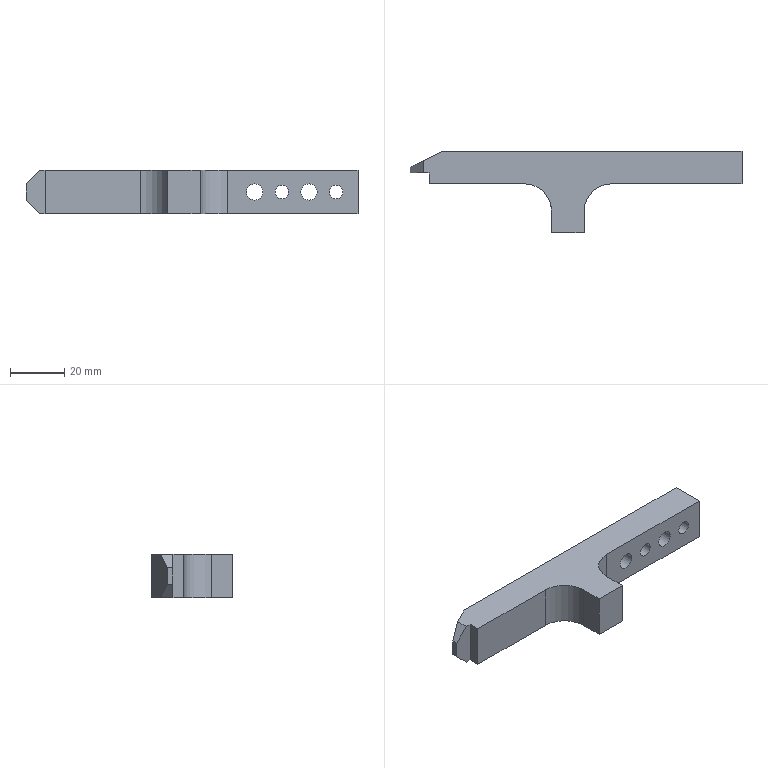Part | NX | features BREP 1 | 1 solid | 21 faces | box 122 x 30 x 16 mm | volume 25322 mm3 | plane 15 | cylinder 6 | commonest cylinder face diameters 5 x2 6 x2 20 x2
STEP:
#1=CARTESIAN_POINT('',(-40.,30.,16.));
#2=VERTEX_POINT('',#1);
#3=CARTESIAN_POINT('',(-40.,30.,0.));
#4=VERTEX_POINT('',#3);
#5=CARTESIAN_POINT('',(-40.,30.,16.));
#6=DIRECTION('',(0.,0.,-1.));
#7=VECTOR('',#6,1000.);
#8=LINE('',#5,#7);
#9=EDGE_CURVE('',#2,#4,#8,.T.);
#10=ORIENTED_EDGE('',*,*,#9,.F.);
#11=CARTESIAN_POINT('',(70.,30.,16.));
#12=VERTEX_POINT('',#11);
#13=CARTESIAN_POINT('',(0.,30.,16.));
#14=DIRECTION('',(-1.,0.,0.));
#15=VECTOR('',#14,1000.);
#16=LINE('',#13,#15);
#17=EDGE_CURVE('',#12,#2,#16,.T.);
#18=ORIENTED_EDGE('',*,*,#17,.F.);
#19=CARTESIAN_POINT('',(70.,30.,0.));
#20=VERTEX_POINT('',#19);
#21=CARTESIAN_POINT('',(70.,30.,16.));
#22=DIRECTION('',(0.,0.,1.));
#23=VECTOR('',#22,1000.);
#24=LINE('',#21,#23);
#25=EDGE_CURVE('',#20,#12,#24,.T.);
#26=ORIENTED_EDGE('',*,*,#25,.F.);
#27=CARTESIAN_POINT('',(0.,30.,0.));
#28=DIRECTION('',(1.,0.,0.));
#29=VECTOR('',#28,1000.);
#30=LINE('',#27,#29);
#31=EDGE_CURVE('',#4,#20,#30,.T.);
#32=ORIENTED_EDGE('',*,*,#31,.F.);
#33=EDGE_LOOP('',(#10,#18,#26,#32));
#34=FACE_BOUND('',#33,.T.);
#35=CARTESIAN_POINT('',(42.,30.,10.5));
#36=VERTEX_POINT('',#35);
#37=CARTESIAN_POINT('',(42.,30.,8.));
#38=DIRECTION('',(0.,1.,0.));
#39=DIRECTION('',(0.,0.,1.));
#40=AXIS2_PLACEMENT_3D('',#37,#38,#39);
#41=CIRCLE('',#40,2.5);
#42=EDGE_CURVE('',#36,#36,#41,.T.);
#43=ORIENTED_EDGE('',*,*,#42,.F.);
#44=EDGE_LOOP('',(#43));
#45=FACE_BOUND('',#44,.T.);
#46=CARTESIAN_POINT('',(62.,30.,10.5));
#47=VERTEX_POINT('',#46);
#48=CARTESIAN_POINT('',(62.,30.,8.));
#49=DIRECTION('',(0.,1.,0.));
#50=DIRECTION('',(0.,0.,1.));
#51=AXIS2_PLACEMENT_3D('',#48,#49,#50);
#52=CIRCLE('',#51,2.5);
#53=EDGE_CURVE('',#47,#47,#52,.T.);
#54=ORIENTED_EDGE('',*,*,#53,.F.);
#55=EDGE_LOOP('',(#54));
#56=FACE_BOUND('',#55,.T.);
#57=CARTESIAN_POINT('',(52.,30.,11.));
#58=VERTEX_POINT('',#57);
#59=CARTESIAN_POINT('',(52.,30.,8.));
#60=DIRECTION('',(0.,1.,0.));
#61=DIRECTION('',(0.,0.,1.));
#62=AXIS2_PLACEMENT_3D('',#59,#60,#61);
#63=CIRCLE('',#62,3.);
#64=EDGE_CURVE('',#58,#58,#63,.T.);
#65=ORIENTED_EDGE('',*,*,#64,.F.);
#66=EDGE_LOOP('',(#65));
#67=FACE_BOUND('',#66,.T.);
#68=CARTESIAN_POINT('',(32.,30.,11.));
#69=VERTEX_POINT('',#68);
#70=CARTESIAN_POINT('',(32.,30.,8.));
#71=DIRECTION('',(0.,1.,0.));
#72=DIRECTION('',(0.,0.,1.));
#73=AXIS2_PLACEMENT_3D('',#70,#71,#72);
#74=CIRCLE('',#73,3.);
#75=EDGE_CURVE('',#69,#69,#74,.T.);
#76=ORIENTED_EDGE('',*,*,#75,.F.);
#77=EDGE_LOOP('',(#76));
#78=FACE_BOUND('',#77,.T.);
#79=CARTESIAN_POINT('',(0.,30.,16.));
#80=DIRECTION('',(0.,-1.,0.));
#81=DIRECTION('',(0.,0.,1.));
#82=AXIS2_PLACEMENT_3D('',#79,#80,#81);
#83=PLANE('',#82);
#84=ADVANCED_FACE('',(#34,#45,#56,#67,#78),#83,.F.);
#85=CARTESIAN_POINT('',(-10.,18.,0.));
#86=VERTEX_POINT('',#85);
#87=CARTESIAN_POINT('',(-45.,18.,0.));
#88=VERTEX_POINT('',#87);
#89=CARTESIAN_POINT('',(0.,18.,0.));
#90=DIRECTION('',(-1.,0.,0.));
#91=VECTOR('',#90,1000.);
#92=LINE('',#89,#91);
#93=EDGE_CURVE('',#86,#88,#92,.T.);
#94=ORIENTED_EDGE('',*,*,#93,.T.);
#95=CARTESIAN_POINT('',(-45.,22.,0.));
#96=VERTEX_POINT('',#95);
#97=CARTESIAN_POINT('',(-45.,0.,0.));
#98=DIRECTION('',(0.,1.,0.));
#99=VECTOR('',#98,1000.);
#100=LINE('',#97,#99);
#101=EDGE_CURVE('',#88,#96,#100,.T.);
#102=ORIENTED_EDGE('',*,*,#101,.T.);
#103=CARTESIAN_POINT('',(-47.,22.,0.));
#104=VERTEX_POINT('',#103);
#105=CARTESIAN_POINT('',(0.,22.,0.));
#106=DIRECTION('',(-1.,0.,0.));
#107=VECTOR('',#106,1000.);
#108=LINE('',#105,#107);
#109=EDGE_CURVE('',#96,#104,#108,.T.);
#110=ORIENTED_EDGE('',*,*,#109,.T.);
#111=CARTESIAN_POINT('',(-47.,26.5,0.));
#112=VERTEX_POINT('',#111);
#113=CARTESIAN_POINT('',(-47.,0.,0.));
#114=DIRECTION('',(0.,1.,0.));
#115=VECTOR('',#114,1000.);
#116=LINE('',#113,#115);
#117=EDGE_CURVE('',#104,#112,#116,.T.);
#118=ORIENTED_EDGE('',*,*,#117,.T.);
#119=CARTESIAN_POINT('',(-47.,26.5,0.));
#120=DIRECTION('',(0.8944,0.4472,0.));
#121=VECTOR('',#120,1000.);
#122=LINE('',#119,#121);
#123=EDGE_CURVE('',#112,#4,#122,.T.);
#124=ORIENTED_EDGE('',*,*,#123,.T.);
#125=ORIENTED_EDGE('',*,*,#31,.T.);
#126=CARTESIAN_POINT('',(70.,18.,0.));
#127=VERTEX_POINT('',#126);
#128=CARTESIAN_POINT('',(70.,0.,0.));
#129=DIRECTION('',(0.,-1.,0.));
#130=VECTOR('',#129,1000.);
#131=LINE('',#128,#130);
#132=EDGE_CURVE('',#20,#127,#131,.T.);
#133=ORIENTED_EDGE('',*,*,#132,.T.);
#134=CARTESIAN_POINT('',(22.,18.,0.));
#135=VERTEX_POINT('',#134);
#136=CARTESIAN_POINT('',(0.,18.,0.));
#137=DIRECTION('',(-1.,0.,0.));
#138=VECTOR('',#137,1000.);
#139=LINE('',#136,#138);
#140=EDGE_CURVE('',#127,#135,#139,.T.);
#141=ORIENTED_EDGE('',*,*,#140,.T.);
#142=CARTESIAN_POINT('',(12.,8.,0.));
#143=VERTEX_POINT('',#142);
#144=CARTESIAN_POINT('',(22.,8.,0.));
#145=DIRECTION('',(0.,0.,1.));
#146=DIRECTION('',(1.,0.,0.));
#147=AXIS2_PLACEMENT_3D('',#144,#145,#146);
#148=CIRCLE('',#147,10.);
#149=EDGE_CURVE('',#135,#143,#148,.T.);
#150=ORIENTED_EDGE('',*,*,#149,.T.);
#151=CARTESIAN_POINT('',(12.,0.,0.));
#152=VERTEX_POINT('',#151);
#153=CARTESIAN_POINT('',(12.,0.,0.));
#154=DIRECTION('',(0.,-1.,0.));
#155=VECTOR('',#154,1000.);
#156=LINE('',#153,#155);
#157=EDGE_CURVE('',#143,#152,#156,.T.);
#158=ORIENTED_EDGE('',*,*,#157,.T.);
#159=CARTESIAN_POINT('',(0.,0.,0.));
#160=VERTEX_POINT('',#159);
#161=CARTESIAN_POINT('',(0.,0.,0.));
#162=DIRECTION('',(-1.,0.,0.));
#163=VECTOR('',#162,1000.);
#164=LINE('',#161,#163);
#165=EDGE_CURVE('',#152,#160,#164,.T.);
#166=ORIENTED_EDGE('',*,*,#165,.T.);
#167=CARTESIAN_POINT('',(0.,8.,0.));
#168=VERTEX_POINT('',#167);
#169=CARTESIAN_POINT('',(0.,0.,0.));
#170=DIRECTION('',(0.,1.,0.));
#171=VECTOR('',#170,1000.);
#172=LINE('',#169,#171);
#173=EDGE_CURVE('',#160,#168,#172,.T.);
#174=ORIENTED_EDGE('',*,*,#173,.T.);
#175=CARTESIAN_POINT('',(-10.,8.,0.));
#176=DIRECTION('',(0.,0.,1.));
#177=DIRECTION('',(1.,0.,0.));
#178=AXIS2_PLACEMENT_3D('',#175,#176,#177);
#179=CIRCLE('',#178,10.);
#180=EDGE_CURVE('',#168,#86,#179,.T.);
#181=ORIENTED_EDGE('',*,*,#180,.T.);
#182=EDGE_LOOP('',(#94,#102,#110,#118,#124,#125,#133,#141,#150,#158,#166,#174,#181));
#183=FACE_BOUND('',#182,.T.);
#184=CARTESIAN_POINT('',(0.,0.,0.));
#185=DIRECTION('',(0.,0.,-1.));
#186=DIRECTION('',(1.,0.,0.));
#187=AXIS2_PLACEMENT_3D('',#184,#185,#186);
#188=PLANE('',#187);
#189=ADVANCED_FACE('',(#183),#188,.T.);
#190=CARTESIAN_POINT('',(-52.,24.,5.));
#191=VERTEX_POINT('',#190);
#192=CARTESIAN_POINT('',(-52.,24.,5.));
#193=DIRECTION('',(0.6667,0.3333,-0.6667));
#194=VECTOR('',#193,1000.);
#195=LINE('',#192,#194);
#196=EDGE_CURVE('',#191,#112,#195,.T.);
#197=ORIENTED_EDGE('',*,*,#196,.F.);
#198=CARTESIAN_POINT('',(-52.,24.,11.));
#199=VERTEX_POINT('',#198);
#200=CARTESIAN_POINT('',(-52.,24.,0.));
#201=DIRECTION('',(0.,0.,-1.));
#202=VECTOR('',#201,1000.);
#203=LINE('',#200,#202);
#204=EDGE_CURVE('',#199,#191,#203,.T.);
#205=ORIENTED_EDGE('',*,*,#204,.F.);
#206=CARTESIAN_POINT('',(-47.,26.5,16.));
#207=VERTEX_POINT('',#206);
#208=CARTESIAN_POINT('',(-47.,26.5,16.));
#209=DIRECTION('',(-0.6667,-0.3333,-0.6667));
#210=VECTOR('',#209,1000.);
#211=LINE('',#208,#210);
#212=EDGE_CURVE('',#207,#199,#211,.T.);
#213=ORIENTED_EDGE('',*,*,#212,.F.);
#214=CARTESIAN_POINT('',(-52.,24.,16.));
#215=DIRECTION('',(-0.8944,-0.4472,0.));
#216=VECTOR('',#215,1000.);
#217=LINE('',#214,#216);
#218=EDGE_CURVE('',#2,#207,#217,.T.);
#219=ORIENTED_EDGE('',*,*,#218,.F.);
#220=ORIENTED_EDGE('',*,*,#9,.T.);
#221=ORIENTED_EDGE('',*,*,#123,.F.);
#222=EDGE_LOOP('',(#197,#205,#213,#219,#220,#221));
#223=FACE_BOUND('',#222,.T.);
#224=CARTESIAN_POINT('',(-52.,24.,0.));
#225=DIRECTION('',(0.4472,-0.8944,0.));
#226=DIRECTION('',(-0.8944,-0.4472,0.));
#227=AXIS2_PLACEMENT_3D('',#224,#225,#226);
#228=PLANE('',#227);
#229=ADVANCED_FACE('',(#223),#228,.F.);
#230=CARTESIAN_POINT('',(-47.,22.,16.));
#231=VERTEX_POINT('',#230);
#232=CARTESIAN_POINT('',(-47.,0.,16.));
#233=DIRECTION('',(0.,1.,0.));
#234=VECTOR('',#233,1000.);
#235=LINE('',#232,#234);
#236=EDGE_CURVE('',#231,#207,#235,.T.);
#237=ORIENTED_EDGE('',*,*,#236,.F.);
#238=CARTESIAN_POINT('',(-45.,22.,16.));
#239=VERTEX_POINT('',#238);
#240=CARTESIAN_POINT('',(0.,22.,16.));
#241=DIRECTION('',(-1.,0.,0.));
#242=VECTOR('',#241,1000.);
#243=LINE('',#240,#242);
#244=EDGE_CURVE('',#239,#231,#243,.T.);
#245=ORIENTED_EDGE('',*,*,#244,.F.);
#246=CARTESIAN_POINT('',(-45.,18.,16.));
#247=VERTEX_POINT('',#246);
#248=CARTESIAN_POINT('',(-45.,0.,16.));
#249=DIRECTION('',(0.,1.,0.));
#250=VECTOR('',#249,1000.);
#251=LINE('',#248,#250);
#252=EDGE_CURVE('',#247,#239,#251,.T.);
#253=ORIENTED_EDGE('',*,*,#252,.F.);
#254=CARTESIAN_POINT('',(-10.,18.,16.));
#255=VERTEX_POINT('',#254);
#256=CARTESIAN_POINT('',(0.,18.,16.));
#257=DIRECTION('',(-1.,0.,0.));
#258=VECTOR('',#257,1000.);
#259=LINE('',#256,#258);
#260=EDGE_CURVE('',#255,#247,#259,.T.);
#261=ORIENTED_EDGE('',*,*,#260,.F.);
#262=CARTESIAN_POINT('',(0.,8.,16.));
#263=VERTEX_POINT('',#262);
#264=CARTESIAN_POINT('',(-10.,8.,16.));
#265=DIRECTION('',(0.,0.,1.));
#266=DIRECTION('',(1.,0.,0.));
#267=AXIS2_PLACEMENT_3D('',#264,#265,#266);
#268=CIRCLE('',#267,10.);
#269=EDGE_CURVE('',#263,#255,#268,.T.);
#270=ORIENTED_EDGE('',*,*,#269,.F.);
#271=CARTESIAN_POINT('',(0.,0.,16.));
#272=VERTEX_POINT('',#271);
#273=CARTESIAN_POINT('',(0.,0.,16.));
#274=DIRECTION('',(0.,1.,0.));
#275=VECTOR('',#274,1000.);
#276=LINE('',#273,#275);
#277=EDGE_CURVE('',#272,#263,#276,.T.);
#278=ORIENTED_EDGE('',*,*,#277,.F.);
#279=CARTESIAN_POINT('',(12.,0.,16.));
#280=VERTEX_POINT('',#279);
#281=CARTESIAN_POINT('',(0.,0.,16.));
#282=DIRECTION('',(-1.,0.,0.));
#283=VECTOR('',#282,1000.);
#284=LINE('',#281,#283);
#285=EDGE_CURVE('',#280,#272,#284,.T.);
#286=ORIENTED_EDGE('',*,*,#285,.F.);
#287=CARTESIAN_POINT('',(12.,8.,16.));
#288=VERTEX_POINT('',#287);
#289=CARTESIAN_POINT('',(12.,0.,16.));
#290=DIRECTION('',(0.,-1.,0.));
#291=VECTOR('',#290,1000.);
#292=LINE('',#289,#291);
#293=EDGE_CURVE('',#288,#280,#292,.T.);
#294=ORIENTED_EDGE('',*,*,#293,.F.);
#295=CARTESIAN_POINT('',(22.,18.,16.));
#296=VERTEX_POINT('',#295);
#297=CARTESIAN_POINT('',(22.,8.,16.));
#298=DIRECTION('',(0.,0.,1.));
#299=DIRECTION('',(1.,0.,0.));
#300=AXIS2_PLACEMENT_3D('',#297,#298,#299);
#301=CIRCLE('',#300,10.);
#302=EDGE_CURVE('',#296,#288,#301,.T.);
#303=ORIENTED_EDGE('',*,*,#302,.F.);
#304=CARTESIAN_POINT('',(70.,18.,16.));
#305=VERTEX_POINT('',#304);
#306=CARTESIAN_POINT('',(0.,18.,16.));
#307=DIRECTION('',(-1.,0.,0.));
#308=VECTOR('',#307,1000.);
#309=LINE('',#306,#308);
#310=EDGE_CURVE('',#305,#296,#309,.T.);
#311=ORIENTED_EDGE('',*,*,#310,.F.);
#312=CARTESIAN_POINT('',(70.,0.,16.));
#313=DIRECTION('',(0.,-1.,0.));
#314=VECTOR('',#313,1000.);
#315=LINE('',#312,#314);
#316=EDGE_CURVE('',#12,#305,#315,.T.);
#317=ORIENTED_EDGE('',*,*,#316,.F.);
#318=ORIENTED_EDGE('',*,*,#17,.T.);
#319=ORIENTED_EDGE('',*,*,#218,.T.);
#320=EDGE_LOOP('',(#237,#245,#253,#261,#270,#278,#286,#294,#303,#311,#317,#318,#319));
#321=FACE_BOUND('',#320,.T.);
#322=CARTESIAN_POINT('',(0.,0.,16.));
#323=DIRECTION('',(0.,0.,-1.));
#324=DIRECTION('',(1.,0.,0.));
#325=AXIS2_PLACEMENT_3D('',#322,#323,#324);
#326=PLANE('',#325);
#327=ADVANCED_FACE('',(#321),#326,.F.);
#328=ORIENTED_EDGE('',*,*,#25,.T.);
#329=ORIENTED_EDGE('',*,*,#316,.T.);
#330=CARTESIAN_POINT('',(70.,18.,16.));
#331=DIRECTION('',(0.,0.,1.));
#332=VECTOR('',#331,1000.);
#333=LINE('',#330,#332);
#334=EDGE_CURVE('',#127,#305,#333,.T.);
#335=ORIENTED_EDGE('',*,*,#334,.F.);
#336=ORIENTED_EDGE('',*,*,#132,.F.);
#337=EDGE_LOOP('',(#328,#329,#335,#336));
#338=FACE_BOUND('',#337,.T.);
#339=CARTESIAN_POINT('',(70.,30.,16.));
#340=DIRECTION('',(-1.,0.,0.));
#341=DIRECTION('',(0.,0.,-1.));
#342=AXIS2_PLACEMENT_3D('',#339,#340,#341);
#343=PLANE('',#342);
#344=ADVANCED_FACE('',(#338),#343,.F.);
#345=CARTESIAN_POINT('',(42.,18.,10.5));
#346=VERTEX_POINT('',#345);
#347=CARTESIAN_POINT('',(42.,18.,8.));
#348=DIRECTION('',(0.,1.,0.));
#349=DIRECTION('',(0.,0.,1.));
#350=AXIS2_PLACEMENT_3D('',#347,#348,#349);
#351=CIRCLE('',#350,2.5);
#352=EDGE_CURVE('',#346,#346,#351,.T.);
#353=ORIENTED_EDGE('',*,*,#352,.F.);
#354=EDGE_LOOP('',(#353));
#355=FACE_BOUND('',#354,.T.);
#356=ORIENTED_EDGE('',*,*,#42,.T.);
#357=EDGE_LOOP('',(#356));
#358=FACE_BOUND('',#357,.T.);
#359=CARTESIAN_POINT('',(42.,30.,8.));
#360=DIRECTION('',(0.,1.,0.));
#361=DIRECTION('',(0.,0.,-1.));
#362=AXIS2_PLACEMENT_3D('',#359,#360,#361);
#363=CYLINDRICAL_SURFACE('',#362,2.5);
#364=ADVANCED_FACE('',(#355,#358),#363,.F.);
#365=CARTESIAN_POINT('',(62.,18.,10.5));
#366=VERTEX_POINT('',#365);
#367=CARTESIAN_POINT('',(62.,18.,8.));
#368=DIRECTION('',(0.,1.,0.));
#369=DIRECTION('',(0.,0.,1.));
#370=AXIS2_PLACEMENT_3D('',#367,#368,#369);
#371=CIRCLE('',#370,2.5);
#372=EDGE_CURVE('',#366,#366,#371,.T.);
#373=ORIENTED_EDGE('',*,*,#372,.F.);
#374=EDGE_LOOP('',(#373));
#375=FACE_BOUND('',#374,.T.);
#376=ORIENTED_EDGE('',*,*,#53,.T.);
#377=EDGE_LOOP('',(#376));
#378=FACE_BOUND('',#377,.T.);
#379=CARTESIAN_POINT('',(62.,30.,8.));
#380=DIRECTION('',(0.,1.,0.));
#381=DIRECTION('',(0.,0.,-1.));
#382=AXIS2_PLACEMENT_3D('',#379,#380,#381);
#383=CYLINDRICAL_SURFACE('',#382,2.5);
#384=ADVANCED_FACE('',(#375,#378),#383,.F.);
#385=CARTESIAN_POINT('',(52.,18.,11.));
#386=VERTEX_POINT('',#385);
#387=CARTESIAN_POINT('',(52.,18.,8.));
#388=DIRECTION('',(0.,1.,0.));
#389=DIRECTION('',(0.,0.,1.));
#390=AXIS2_PLACEMENT_3D('',#387,#388,#389);
#391=CIRCLE('',#390,3.);
#392=EDGE_CURVE('',#386,#386,#391,.T.);
#393=ORIENTED_EDGE('',*,*,#392,.F.);
#394=EDGE_LOOP('',(#393));
#395=FACE_BOUND('',#394,.T.);
#396=ORIENTED_EDGE('',*,*,#64,.T.);
#397=EDGE_LOOP('',(#396));
#398=FACE_BOUND('',#397,.T.);
#399=CARTESIAN_POINT('',(52.,30.,8.));
#400=DIRECTION('',(0.,1.,0.));
#401=DIRECTION('',(0.,0.,-1.));
#402=AXIS2_PLACEMENT_3D('',#399,#400,#401);
#403=CYLINDRICAL_SURFACE('',#402,3.);
#404=ADVANCED_FACE('',(#395,#398),#403,.F.);
#405=CARTESIAN_POINT('',(32.,18.,11.));
#406=VERTEX_POINT('',#405);
#407=CARTESIAN_POINT('',(32.,18.,8.));
#408=DIRECTION('',(0.,1.,0.));
#409=DIRECTION('',(0.,0.,1.));
#410=AXIS2_PLACEMENT_3D('',#407,#408,#409);
#411=CIRCLE('',#410,3.);
#412=EDGE_CURVE('',#406,#406,#411,.T.);
#413=ORIENTED_EDGE('',*,*,#412,.F.);
#414=EDGE_LOOP('',(#413));
#415=FACE_BOUND('',#414,.T.);
#416=ORIENTED_EDGE('',*,*,#75,.T.);
#417=EDGE_LOOP('',(#416));
#418=FACE_BOUND('',#417,.T.);
#419=CARTESIAN_POINT('',(32.,30.,8.));
#420=DIRECTION('',(0.,1.,0.));
#421=DIRECTION('',(0.,0.,-1.));
#422=AXIS2_PLACEMENT_3D('',#419,#420,#421);
#423=CYLINDRICAL_SURFACE('',#422,3.);
#424=ADVANCED_FACE('',(#415,#418),#423,.F.);
#425=ORIENTED_EDGE('',*,*,#101,.F.);
#426=CARTESIAN_POINT('',(-45.,18.,0.));
#427=DIRECTION('',(0.,0.,1.));
#428=VECTOR('',#427,1000.);
#429=LINE('',#426,#428);
#430=EDGE_CURVE('',#88,#247,#429,.T.);
#431=ORIENTED_EDGE('',*,*,#430,.T.);
#432=ORIENTED_EDGE('',*,*,#252,.T.);
#433=CARTESIAN_POINT('',(-45.,22.,0.));
#434=DIRECTION('',(0.,0.,-1.));
#435=VECTOR('',#434,1000.);
#436=LINE('',#433,#435);
#437=EDGE_CURVE('',#239,#96,#436,.T.);
#438=ORIENTED_EDGE('',*,*,#437,.T.);
#439=EDGE_LOOP('',(#425,#431,#432,#438));
#440=FACE_BOUND('',#439,.T.);
#441=CARTESIAN_POINT('',(-45.,22.,0.));
#442=DIRECTION('',(-1.,0.,0.));
#443=DIRECTION('',(0.,0.,-1.));
#444=AXIS2_PLACEMENT_3D('',#441,#442,#443);
#445=PLANE('',#444);
#446=ADVANCED_FACE('',(#440),#445,.T.);
#447=ORIENTED_EDGE('',*,*,#260,.T.);
#448=ORIENTED_EDGE('',*,*,#430,.F.);
#449=ORIENTED_EDGE('',*,*,#93,.F.);
#450=CARTESIAN_POINT('',(-10.,18.,0.));
#451=DIRECTION('',(0.,0.,1.));
#452=VECTOR('',#451,1000.);
#453=LINE('',#450,#452);
#454=EDGE_CURVE('',#86,#255,#453,.T.);
#455=ORIENTED_EDGE('',*,*,#454,.T.);
#456=EDGE_LOOP('',(#447,#448,#449,#455));
#457=FACE_BOUND('',#456,.T.);
#458=CARTESIAN_POINT('',(-45.,18.,0.));
#459=DIRECTION('',(0.,-1.,0.));
#460=DIRECTION('',(0.,0.,1.));
#461=AXIS2_PLACEMENT_3D('',#458,#459,#460);
#462=PLANE('',#461);
#463=ADVANCED_FACE('',(#457),#462,.T.);
#464=CARTESIAN_POINT('',(0.,8.,0.));
#465=DIRECTION('',(0.,0.,-1.));
#466=VECTOR('',#465,1000.);
#467=LINE('',#464,#466);
#468=EDGE_CURVE('',#263,#168,#467,.T.);
#469=ORIENTED_EDGE('',*,*,#468,.F.);
#470=ORIENTED_EDGE('',*,*,#269,.T.);
#471=ORIENTED_EDGE('',*,*,#454,.F.);
#472=ORIENTED_EDGE('',*,*,#180,.F.);
#473=EDGE_LOOP('',(#469,#470,#471,#472));
#474=FACE_BOUND('',#473,.T.);
#475=CARTESIAN_POINT('',(-10.,8.,0.));
#476=DIRECTION('',(0.,0.,1.));
#477=DIRECTION('',(-1.,0.,0.));
#478=AXIS2_PLACEMENT_3D('',#475,#476,#477);
#479=CYLINDRICAL_SURFACE('',#478,10.);
#480=ADVANCED_FACE('',(#474),#479,.F.);
#481=ORIENTED_EDGE('',*,*,#468,.T.);
#482=ORIENTED_EDGE('',*,*,#173,.F.);
#483=CARTESIAN_POINT('',(0.,0.,16.));
#484=DIRECTION('',(0.,0.,-1.));
#485=VECTOR('',#484,1000.);
#486=LINE('',#483,#485);
#487=EDGE_CURVE('',#272,#160,#486,.T.);
#488=ORIENTED_EDGE('',*,*,#487,.F.);
#489=ORIENTED_EDGE('',*,*,#277,.T.);
#490=EDGE_LOOP('',(#481,#482,#488,#489));
#491=FACE_BOUND('',#490,.T.);
#492=CARTESIAN_POINT('',(0.,0.,16.));
#493=DIRECTION('',(1.,0.,0.));
#494=DIRECTION('',(0.,0.,1.));
#495=AXIS2_PLACEMENT_3D('',#492,#493,#494);
#496=PLANE('',#495);
#497=ADVANCED_FACE('',(#491),#496,.F.);
#498=CARTESIAN_POINT('',(12.,0.,16.));
#499=DIRECTION('',(0.,0.,-1.));
#500=VECTOR('',#499,1000.);
#501=LINE('',#498,#500);
#502=EDGE_CURVE('',#280,#152,#501,.T.);
#503=ORIENTED_EDGE('',*,*,#502,.F.);
#504=ORIENTED_EDGE('',*,*,#285,.T.);
#505=ORIENTED_EDGE('',*,*,#487,.T.);
#506=ORIENTED_EDGE('',*,*,#165,.F.);
#507=EDGE_LOOP('',(#503,#504,#505,#506));
#508=FACE_BOUND('',#507,.T.);
#509=CARTESIAN_POINT('',(12.,0.,16.));
#510=DIRECTION('',(0.,1.,0.));
#511=DIRECTION('',(1.,0.,0.));
#512=AXIS2_PLACEMENT_3D('',#509,#510,#511);
#513=PLANE('',#512);
#514=ADVANCED_FACE('',(#508),#513,.F.);
#515=CARTESIAN_POINT('',(12.,8.,16.));
#516=DIRECTION('',(0.,0.,-1.));
#517=VECTOR('',#516,1000.);
#518=LINE('',#515,#517);
#519=EDGE_CURVE('',#288,#143,#518,.T.);
#520=ORIENTED_EDGE('',*,*,#519,.F.);
#521=ORIENTED_EDGE('',*,*,#293,.T.);
#522=ORIENTED_EDGE('',*,*,#502,.T.);
#523=ORIENTED_EDGE('',*,*,#157,.F.);
#524=EDGE_LOOP('',(#520,#521,#522,#523));
#525=FACE_BOUND('',#524,.T.);
#526=CARTESIAN_POINT('',(12.,18.,16.));
#527=DIRECTION('',(-1.,0.,0.));
#528=DIRECTION('',(0.,1.,0.));
#529=AXIS2_PLACEMENT_3D('',#526,#527,#528);
#530=PLANE('',#529);
#531=ADVANCED_FACE('',(#525),#530,.F.);
#532=ORIENTED_EDGE('',*,*,#519,.T.);
#533=ORIENTED_EDGE('',*,*,#149,.F.);
#534=CARTESIAN_POINT('',(22.,18.,16.));
#535=DIRECTION('',(0.,0.,-1.));
#536=VECTOR('',#535,1000.);
#537=LINE('',#534,#536);
#538=EDGE_CURVE('',#296,#135,#537,.T.);
#539=ORIENTED_EDGE('',*,*,#538,.F.);
#540=ORIENTED_EDGE('',*,*,#302,.T.);
#541=EDGE_LOOP('',(#532,#533,#539,#540));
#542=FACE_BOUND('',#541,.T.);
#543=CARTESIAN_POINT('',(22.,8.,16.));
#544=DIRECTION('',(0.,0.,1.));
#545=DIRECTION('',(-1.,0.,0.));
#546=AXIS2_PLACEMENT_3D('',#543,#544,#545);
#547=CYLINDRICAL_SURFACE('',#546,10.);
#548=ADVANCED_FACE('',(#542),#547,.F.);
#549=ORIENTED_EDGE('',*,*,#538,.T.);
#550=ORIENTED_EDGE('',*,*,#140,.F.);
#551=ORIENTED_EDGE('',*,*,#334,.T.);
#552=ORIENTED_EDGE('',*,*,#310,.T.);
#553=EDGE_LOOP('',(#549,#550,#551,#552));
#554=FACE_BOUND('',#553,.T.);
#555=ORIENTED_EDGE('',*,*,#352,.T.);
#556=EDGE_LOOP('',(#555));
#557=FACE_BOUND('',#556,.T.);
#558=ORIENTED_EDGE('',*,*,#372,.T.);
#559=EDGE_LOOP('',(#558));
#560=FACE_BOUND('',#559,.T.);
#561=ORIENTED_EDGE('',*,*,#392,.T.);
#562=EDGE_LOOP('',(#561));
#563=FACE_BOUND('',#562,.T.);
#564=ORIENTED_EDGE('',*,*,#412,.T.);
#565=EDGE_LOOP('',(#564));
#566=FACE_BOUND('',#565,.T.);
#567=CARTESIAN_POINT('',(70.,18.,16.));
#568=DIRECTION('',(0.,1.,0.));
#569=DIRECTION('',(1.,0.,0.));
#570=AXIS2_PLACEMENT_3D('',#567,#568,#569);
#571=PLANE('',#570);
#572=ADVANCED_FACE('',(#554,#557,#560,#563,#566),#571,.F.);
#573=ORIENTED_EDGE('',*,*,#117,.F.);
#574=CARTESIAN_POINT('',(-52.,22.,5.));
#575=VERTEX_POINT('',#574);
#576=CARTESIAN_POINT('',(-52.,22.,5.));
#577=DIRECTION('',(0.7071,0.,-0.7071));
#578=VECTOR('',#577,1000.);
#579=LINE('',#576,#578);
#580=EDGE_CURVE('',#575,#104,#579,.T.);
#581=ORIENTED_EDGE('',*,*,#580,.F.);
#582=CARTESIAN_POINT('',(-52.,30.,5.));
#583=DIRECTION('',(0.,-1.,0.));
#584=VECTOR('',#583,1000.);
#585=LINE('',#582,#584);
#586=EDGE_CURVE('',#191,#575,#585,.T.);
#587=ORIENTED_EDGE('',*,*,#586,.F.);
#588=ORIENTED_EDGE('',*,*,#196,.T.);
#589=EDGE_LOOP('',(#573,#581,#587,#588));
#590=FACE_BOUND('',#589,.T.);
#591=CARTESIAN_POINT('',(-52.,30.,5.));
#592=DIRECTION('',(0.7071,0.,0.7071));
#593=DIRECTION('',(-0.7071,0.,0.7071));
#594=AXIS2_PLACEMENT_3D('',#591,#592,#593);
#595=PLANE('',#594);
#596=ADVANCED_FACE('',(#590),#595,.F.);
#597=ORIENTED_EDGE('',*,*,#244,.T.);
#598=CARTESIAN_POINT('',(-52.,22.,11.));
#599=VERTEX_POINT('',#598);
#600=CARTESIAN_POINT('',(-47.,22.,16.));
#601=DIRECTION('',(-0.7071,0.,-0.7071));
#602=VECTOR('',#601,1000.);
#603=LINE('',#600,#602);
#604=EDGE_CURVE('',#231,#599,#603,.T.);
#605=ORIENTED_EDGE('',*,*,#604,.T.);
#606=CARTESIAN_POINT('',(-52.,22.,0.));
#607=DIRECTION('',(0.,0.,-1.));
#608=VECTOR('',#607,1000.);
#609=LINE('',#606,#608);
#610=EDGE_CURVE('',#599,#575,#609,.T.);
#611=ORIENTED_EDGE('',*,*,#610,.T.);
#612=ORIENTED_EDGE('',*,*,#580,.T.);
#613=ORIENTED_EDGE('',*,*,#109,.F.);
#614=ORIENTED_EDGE('',*,*,#437,.F.);
#615=EDGE_LOOP('',(#597,#605,#611,#612,#613,#614));
#616=FACE_BOUND('',#615,.T.);
#617=CARTESIAN_POINT('',(-52.,22.,0.));
#618=DIRECTION('',(0.,-1.,0.));
#619=DIRECTION('',(0.,0.,1.));
#620=AXIS2_PLACEMENT_3D('',#617,#618,#619);
#621=PLANE('',#620);
#622=ADVANCED_FACE('',(#616),#621,.T.);
#623=ORIENTED_EDGE('',*,*,#610,.F.);
#624=CARTESIAN_POINT('',(-52.,30.,11.));
#625=DIRECTION('',(0.,1.,0.));
#626=VECTOR('',#625,1000.);
#627=LINE('',#624,#626);
#628=EDGE_CURVE('',#599,#199,#627,.T.);
#629=ORIENTED_EDGE('',*,*,#628,.T.);
#630=ORIENTED_EDGE('',*,*,#204,.T.);
#631=ORIENTED_EDGE('',*,*,#586,.T.);
#632=EDGE_LOOP('',(#623,#629,#630,#631));
#633=FACE_BOUND('',#632,.T.);
#634=CARTESIAN_POINT('',(-52.,30.,0.));
#635=DIRECTION('',(-1.,0.,0.));
#636=DIRECTION('',(0.,1.,0.));
#637=AXIS2_PLACEMENT_3D('',#634,#635,#636);
#638=PLANE('',#637);
#639=ADVANCED_FACE('',(#633),#638,.T.);
#640=ORIENTED_EDGE('',*,*,#604,.F.);
#641=ORIENTED_EDGE('',*,*,#236,.T.);
#642=ORIENTED_EDGE('',*,*,#212,.T.);
#643=ORIENTED_EDGE('',*,*,#628,.F.);
#644=EDGE_LOOP('',(#640,#641,#642,#643));
#645=FACE_BOUND('',#644,.T.);
#646=CARTESIAN_POINT('',(-47.,0.,16.));
#647=DIRECTION('',(-0.7071,0.,0.7071));
#648=DIRECTION('',(-0.7071,0.,-0.7071));
#649=AXIS2_PLACEMENT_3D('',#646,#647,#648);
#650=PLANE('',#649);
#651=ADVANCED_FACE('',(#645),#650,.T.);
#652=CLOSED_SHELL('',(#84,#189,#229,#327,#344,#364,#384,#404,#424,#446,#463,#480,#497,#514,#531,#548,#572,#596,#622,#639,#651));
#653=MANIFOLD_SOLID_BREP('',#652);
#654=(LENGTH_UNIT()NAMED_UNIT(*)SI_UNIT(.MILLI.,.METRE.));
#655=UNCERTAINTY_MEASURE_WITH_UNIT(LENGTH_MEASURE(0.00001),#654,'','');
#656=(NAMED_UNIT(*)PLANE_ANGLE_UNIT()SI_UNIT($,.RADIAN.));
#657=(NAMED_UNIT(*)SI_UNIT($,.STERADIAN.)SOLID_ANGLE_UNIT());
#658=(GEOMETRIC_REPRESENTATION_CONTEXT(3)GLOBAL_UNCERTAINTY_ASSIGNED_CONTEXT((#655))GLOBAL_UNIT_ASSIGNED_CONTEXT((#654,#656,#657))REPRESENTATION_CONTEXT('',''));
#659=ADVANCED_BREP_SHAPE_REPRESENTATION('',(#653),#658);